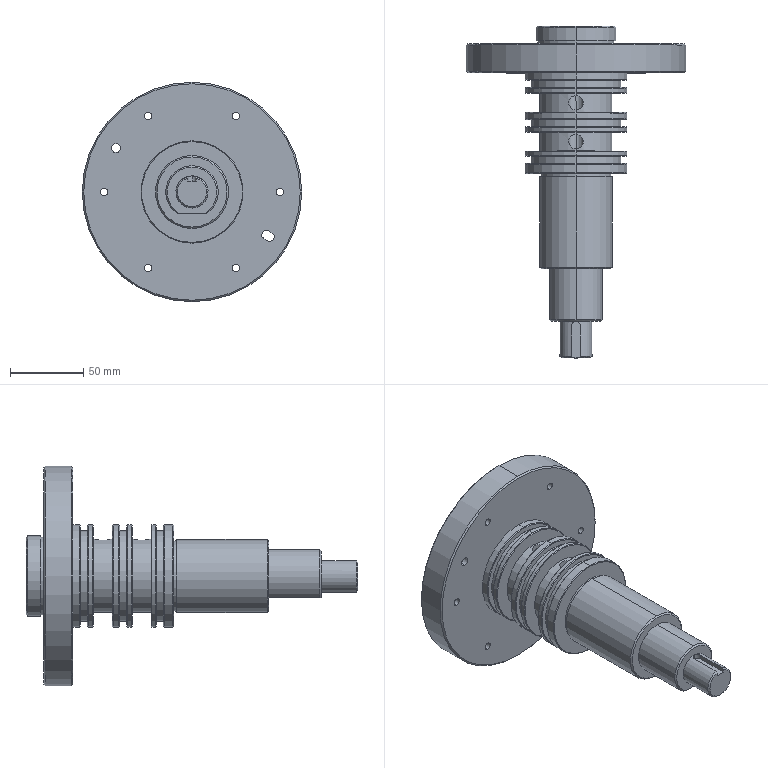Part | STEP file | 10-05 rotary shaft | 1 solid | 144 faces | box 150 x 227 x 150 mm | volume 734165 mm3 | cylinder 71 | cone 43 | plane 30 | commonest cylinder face diameters 5 x12 70 x12 10 x8 6 x7 50 x6 62 x6